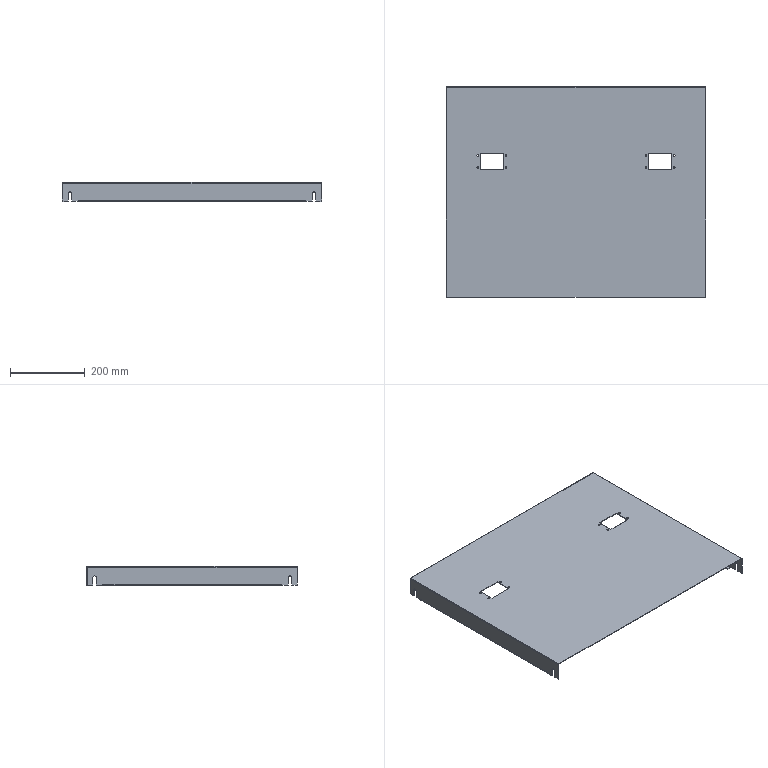Part | SolidWorks | features BaseBody 1 | 1 solid | 132 faces | box 695 x 563.5 x 51.5 mm | volume 732855 mm3 | plane 88 | cylinder 40 | spline 4 | commonest cylinder face diameters 4.5 x16 9 x12 1.473 x6 4.473 x6